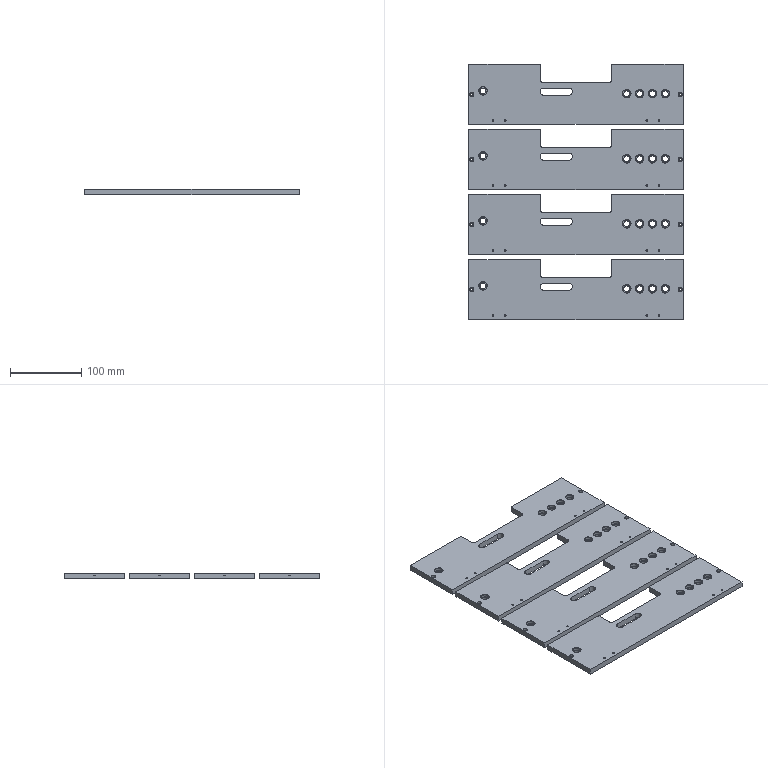CAM job | NX | 3-axis milling | part box 300 x 357 x 8 mm | stock box 304 x 361 x 8 mm
Tools:
number,name,description,diameter,corner_radius,flute_length,length,flutes
2,D4A45,Milling Tool-5 Parameters,4.0,0.0,2.0,2.0,2
6,D6,Milling Tool-5 Parameters,6.0,0.0,50.0,75.0,2
4,D4,Milling Tool-5 Parameters,4.0,0.0,50.0,75.0,2
12,D2,Milling Tool-5 Parameters,2.0,0.0,50.0,75.0,2
15,D1.5,Milling Tool-5 Parameters,1.5,0.0,50.0,75.0,2
Operations:
program,operation,operation_type,tool,method,geometry_group,spindle_rpm,surface_speed,feed_per_tooth,feed_cut,feed_plunge,cut_length_mm,path_length_mm,cut_time_min,machine_time_min
1吸,ZLEVEL_PROFILE_1_COPY_1_COPY_COPY,ZLevelMilling,D4A45,METHOD,A,9500.0,179.0,0.0526,1000.0,100.0,4640.143,14110.795,4.64,5.587
1吸,ZLEVEL_PROFILE_COPY_COPY_1_COPY,ZLevelMilling,D6,METHOD,A,9500.0,179.0,0.1158,2200.0,1000.0,53591.854,54186.801,24.442,24.502
1吸,ZLEVEL_PROFILE_COPY_COPY_1_COPY_COPY,ZLevelMilling,D6,METHOD,A,9500.0,179.0,0.0868,1650.0,1000.0,5551.088,6083.018,3.424,3.477
1吸,HOLE_MILLING_COPY,CylinderMilling,D6,METHOD,A,9500.0,179.0,0.0789,1500.0,100.0,4006.676,6239.716,2.671,2.894
1吸,HOLE_MILLING_COPY_COPY_2,CylinderMilling,D6,METHOD,A,9500.0,179.0,0.0789,1500.0,100.0,1635.478,4025.518,1.09,1.329
1吸,HOLE_MILLING,CylinderMilling,D4,METHOD,A,9500.0,179.0,0.0789,1500.0,100.0,579.071,2524.071,0.386,0.5805
1吸,HOLE_MILLING_COPY_2,CylinderMilling,D2,METHOD,A,9500.0,59.0,0.0526,1000.0,100.0,1276.104,2680.904,1.276,1.417
1吸,HOLE_MILLING_COPY_COPY_1,CylinderMilling,D1.5,METHOD,A,9500.0,44.0,0.0368,700.0,100.0,2876.698,5332.081,4.11,4.355
1吸,ZLEVEL_PROFILE_COPY_COPY_COPY_COPY_COPY,ZLevelMilling,D4,MILL_FINISH,A,9500.0,119.0,0.0632,1200.0,1000.0,3321.222,4067.061,2.769,2.844